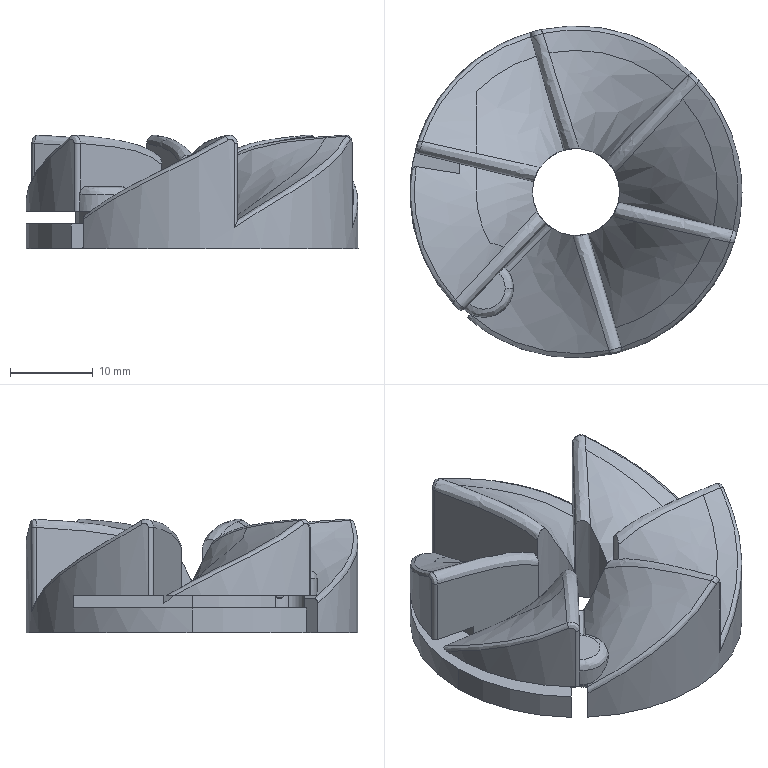Part | SolidWorks | features BaseBody 1 | 1 solid | 101 faces | box 40.118 x 40.118 x 13.737 mm | volume 8402 mm3 | spline 42 | cylinder 35 | plane 24 | commonest cylinder face diameters 1.003 x8 16.413 x6 34.235 x6 40.118 x4 4.062 x3 7.071 x2